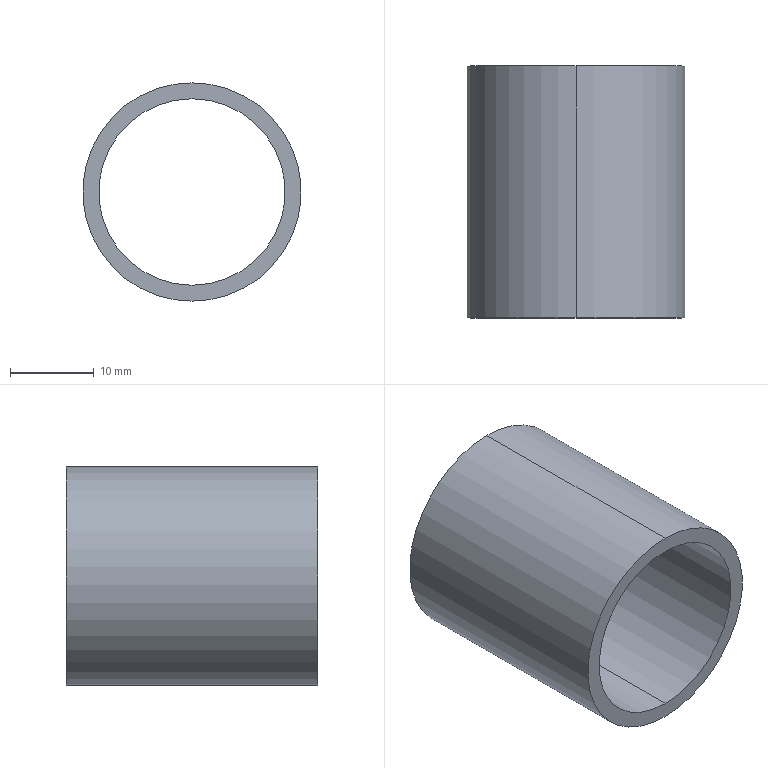Part | SolidWorks | features BaseBody 1 | 1 solid | 6 faces | box 26 x 30 x 26 mm | volume 4316 mm3 | cylinder 4 | plane 2 | commonest cylinder face diameters 22.2 x2 26 x2
STEP:
#1=CARTESIAN_POINT('',(0.,-27.,-13.));
#2=VERTEX_POINT('',#1);
#3=CARTESIAN_POINT('',(0.,-27.,13.));
#4=VERTEX_POINT('',#3);
#5=CARTESIAN_POINT('',(0.,-27.,0.));
#6=DIRECTION('',(0.,-1.,0.));
#7=DIRECTION('',(0.,0.,-1.));
#8=AXIS2_PLACEMENT_3D('',#5,#6,#7);
#9=CIRCLE('',#8,13.);
#10=EDGE_CURVE('',#2,#4,#9,.T.);
#11=ORIENTED_EDGE('',*,*,#10,.T.);
#12=CARTESIAN_POINT('',(0.,-57.,13.));
#13=VERTEX_POINT('',#12);
#14=CARTESIAN_POINT('',(0.,-42.,13.));
#15=DIRECTION('',(0.,-1.,0.));
#16=VECTOR('',#15,1000.);
#17=LINE('',#14,#16);
#18=EDGE_CURVE('',#4,#13,#17,.T.);
#19=ORIENTED_EDGE('',*,*,#18,.T.);
#20=CARTESIAN_POINT('',(0.,-57.,-13.));
#21=VERTEX_POINT('',#20);
#22=CARTESIAN_POINT('',(0.,-57.,0.));
#23=DIRECTION('',(0.,1.,0.));
#24=DIRECTION('',(0.,0.,-1.));
#25=AXIS2_PLACEMENT_3D('',#22,#23,#24);
#26=CIRCLE('',#25,13.);
#27=EDGE_CURVE('',#13,#21,#26,.T.);
#28=ORIENTED_EDGE('',*,*,#27,.T.);
#29=CARTESIAN_POINT('',(0.,-42.,-13.));
#30=DIRECTION('',(0.,-1.,0.));
#31=VECTOR('',#30,1000.);
#32=LINE('',#29,#31);
#33=EDGE_CURVE('',#2,#21,#32,.T.);
#34=ORIENTED_EDGE('',*,*,#33,.F.);
#35=EDGE_LOOP('',(#11,#19,#28,#34));
#36=FACE_OUTER_BOUND('',#35,.T.);
#37=CARTESIAN_POINT('',(0.,-42.,0.));
#38=DIRECTION('',(0.,-1.,0.));
#39=DIRECTION('',(0.,0.,-1.));
#40=AXIS2_PLACEMENT_3D('',#37,#38,#39);
#41=CYLINDRICAL_SURFACE('',#40,13.);
#42=ADVANCED_FACE('',(#36),#41,.T.);
#43=CARTESIAN_POINT('',(0.,-27.,11.1));
#44=VERTEX_POINT('',#43);
#45=CARTESIAN_POINT('',(0.,-27.,-11.1));
#46=VERTEX_POINT('',#45);
#47=CARTESIAN_POINT('',(0.,-27.,0.));
#48=DIRECTION('',(0.,-1.,0.));
#49=DIRECTION('',(0.,0.,-1.));
#50=AXIS2_PLACEMENT_3D('',#47,#48,#49);
#51=CIRCLE('',#50,11.1);
#52=EDGE_CURVE('',#44,#46,#51,.T.);
#53=ORIENTED_EDGE('',*,*,#52,.F.);
#54=CARTESIAN_POINT('',(0.,-57.,11.1));
#55=VERTEX_POINT('',#54);
#56=CARTESIAN_POINT('',(0.,-42.,11.1));
#57=DIRECTION('',(0.,-1.,0.));
#58=VECTOR('',#57,1000.);
#59=LINE('',#56,#58);
#60=EDGE_CURVE('',#44,#55,#59,.T.);
#61=ORIENTED_EDGE('',*,*,#60,.T.);
#62=CARTESIAN_POINT('',(0.,-57.,-11.1));
#63=VERTEX_POINT('',#62);
#64=CARTESIAN_POINT('',(0.,-57.,0.));
#65=DIRECTION('',(0.,1.,0.));
#66=DIRECTION('',(0.,0.,-1.));
#67=AXIS2_PLACEMENT_3D('',#64,#65,#66);
#68=CIRCLE('',#67,11.1);
#69=EDGE_CURVE('',#63,#55,#68,.T.);
#70=ORIENTED_EDGE('',*,*,#69,.F.);
#71=CARTESIAN_POINT('',(0.,-42.,-11.1));
#72=DIRECTION('',(0.,-1.,0.));
#73=VECTOR('',#72,1000.);
#74=LINE('',#71,#73);
#75=EDGE_CURVE('',#46,#63,#74,.T.);
#76=ORIENTED_EDGE('',*,*,#75,.F.);
#77=EDGE_LOOP('',(#53,#61,#70,#76));
#78=FACE_OUTER_BOUND('',#77,.T.);
#79=CARTESIAN_POINT('',(0.,-42.,0.));
#80=DIRECTION('',(0.,-1.,0.));
#81=DIRECTION('',(0.,0.,-1.));
#82=AXIS2_PLACEMENT_3D('',#79,#80,#81);
#83=CYLINDRICAL_SURFACE('',#82,11.1);
#84=ADVANCED_FACE('',(#78),#83,.F.);
#85=ORIENTED_EDGE('',*,*,#69,.T.);
#86=CARTESIAN_POINT('',(0.,-57.,0.));
#87=DIRECTION('',(0.,1.,0.));
#88=DIRECTION('',(0.,0.,-1.));
#89=AXIS2_PLACEMENT_3D('',#86,#87,#88);
#90=CIRCLE('',#89,11.1);
#91=EDGE_CURVE('',#55,#63,#90,.T.);
#92=ORIENTED_EDGE('',*,*,#91,.T.);
#93=EDGE_LOOP('',(#85,#92));
#94=FACE_BOUND('',#93,.T.);
#95=CARTESIAN_POINT('',(0.,-57.,0.));
#96=DIRECTION('',(0.,1.,0.));
#97=DIRECTION('',(0.,0.,-1.));
#98=AXIS2_PLACEMENT_3D('',#95,#96,#97);
#99=CIRCLE('',#98,13.);
#100=EDGE_CURVE('',#21,#13,#99,.T.);
#101=ORIENTED_EDGE('',*,*,#100,.F.);
#102=ORIENTED_EDGE('',*,*,#27,.F.);
#103=EDGE_LOOP('',(#101,#102));
#104=FACE_OUTER_BOUND('',#103,.T.);
#105=CARTESIAN_POINT('',(0.,-57.,-12.05));
#106=DIRECTION('',(0.,-1.,0.));
#107=DIRECTION('',(0.,0.,-1.));
#108=AXIS2_PLACEMENT_3D('',#105,#106,#107);
#109=PLANE('',#108);
#110=ADVANCED_FACE('',(#94,#104),#109,.T.);
#111=CARTESIAN_POINT('',(0.,-27.,0.));
#112=DIRECTION('',(0.,-1.,0.));
#113=DIRECTION('',(0.,0.,-1.));
#114=AXIS2_PLACEMENT_3D('',#111,#112,#113);
#115=CIRCLE('',#114,11.1);
#116=EDGE_CURVE('',#46,#44,#115,.T.);
#117=ORIENTED_EDGE('',*,*,#116,.T.);
#118=ORIENTED_EDGE('',*,*,#52,.T.);
#119=EDGE_LOOP('',(#117,#118));
#120=FACE_BOUND('',#119,.T.);
#121=ORIENTED_EDGE('',*,*,#10,.F.);
#122=CARTESIAN_POINT('',(0.,-27.,0.));
#123=DIRECTION('',(0.,-1.,0.));
#124=DIRECTION('',(0.,0.,-1.));
#125=AXIS2_PLACEMENT_3D('',#122,#123,#124);
#126=CIRCLE('',#125,13.);
#127=EDGE_CURVE('',#4,#2,#126,.T.);
#128=ORIENTED_EDGE('',*,*,#127,.F.);
#129=EDGE_LOOP('',(#121,#128));
#130=FACE_OUTER_BOUND('',#129,.T.);
#131=CARTESIAN_POINT('',(0.,-27.,-12.05));
#132=DIRECTION('',(0.,1.,0.));
#133=DIRECTION('',(1.,0.,0.));
#134=AXIS2_PLACEMENT_3D('',#131,#132,#133);
#135=PLANE('',#134);
#136=ADVANCED_FACE('',(#120,#130),#135,.T.);
#137=ORIENTED_EDGE('',*,*,#60,.F.);
#138=ORIENTED_EDGE('',*,*,#116,.F.);
#139=ORIENTED_EDGE('',*,*,#75,.T.);
#140=ORIENTED_EDGE('',*,*,#91,.F.);
#141=EDGE_LOOP('',(#137,#138,#139,#140));
#142=FACE_OUTER_BOUND('',#141,.T.);
#143=CARTESIAN_POINT('',(0.,-42.,0.));
#144=DIRECTION('',(0.,-1.,0.));
#145=DIRECTION('',(0.,0.,-1.));
#146=AXIS2_PLACEMENT_3D('',#143,#144,#145);
#147=CYLINDRICAL_SURFACE('',#146,11.1);
#148=ADVANCED_FACE('',(#142),#147,.F.);
#149=ORIENTED_EDGE('',*,*,#18,.F.);
#150=ORIENTED_EDGE('',*,*,#127,.T.);
#151=ORIENTED_EDGE('',*,*,#33,.T.);
#152=ORIENTED_EDGE('',*,*,#100,.T.);
#153=EDGE_LOOP('',(#149,#150,#151,#152));
#154=FACE_OUTER_BOUND('',#153,.T.);
#155=CARTESIAN_POINT('',(0.,-42.,0.));
#156=DIRECTION('',(0.,-1.,0.));
#157=DIRECTION('',(0.,0.,-1.));
#158=AXIS2_PLACEMENT_3D('',#155,#156,#157);
#159=CYLINDRICAL_SURFACE('',#158,13.);
#160=ADVANCED_FACE('',(#154),#159,.T.);
#161=CLOSED_SHELL('',(#42,#84,#110,#136,#148,#160));
#162=MANIFOLD_SOLID_BREP('',#161);
#163=CARTESIAN_POINT('',(0.,0.,0.));
#164=DIRECTION('',(0.,0.,1.));
#165=DIRECTION('',(1.,0.,0.));
#166=AXIS2_PLACEMENT_3D('',#163,#164,#165);
#167=(LENGTH_UNIT()NAMED_UNIT(*)SI_UNIT(.MILLI.,.METRE.));
#168=UNCERTAINTY_MEASURE_WITH_UNIT(LENGTH_MEASURE(0.00001),#167,'','');
#169=(NAMED_UNIT(*)PLANE_ANGLE_UNIT()SI_UNIT($,.RADIAN.));
#170=(NAMED_UNIT(*)SI_UNIT($,.STERADIAN.)SOLID_ANGLE_UNIT());
#171=(GEOMETRIC_REPRESENTATION_CONTEXT(3)GLOBAL_UNCERTAINTY_ASSIGNED_CONTEXT((#168))GLOBAL_UNIT_ASSIGNED_CONTEXT((#167,#169,#170))REPRESENTATION_CONTEXT('',''));
#172=ADVANCED_BREP_SHAPE_REPRESENTATION('',(#162,#166),#171);